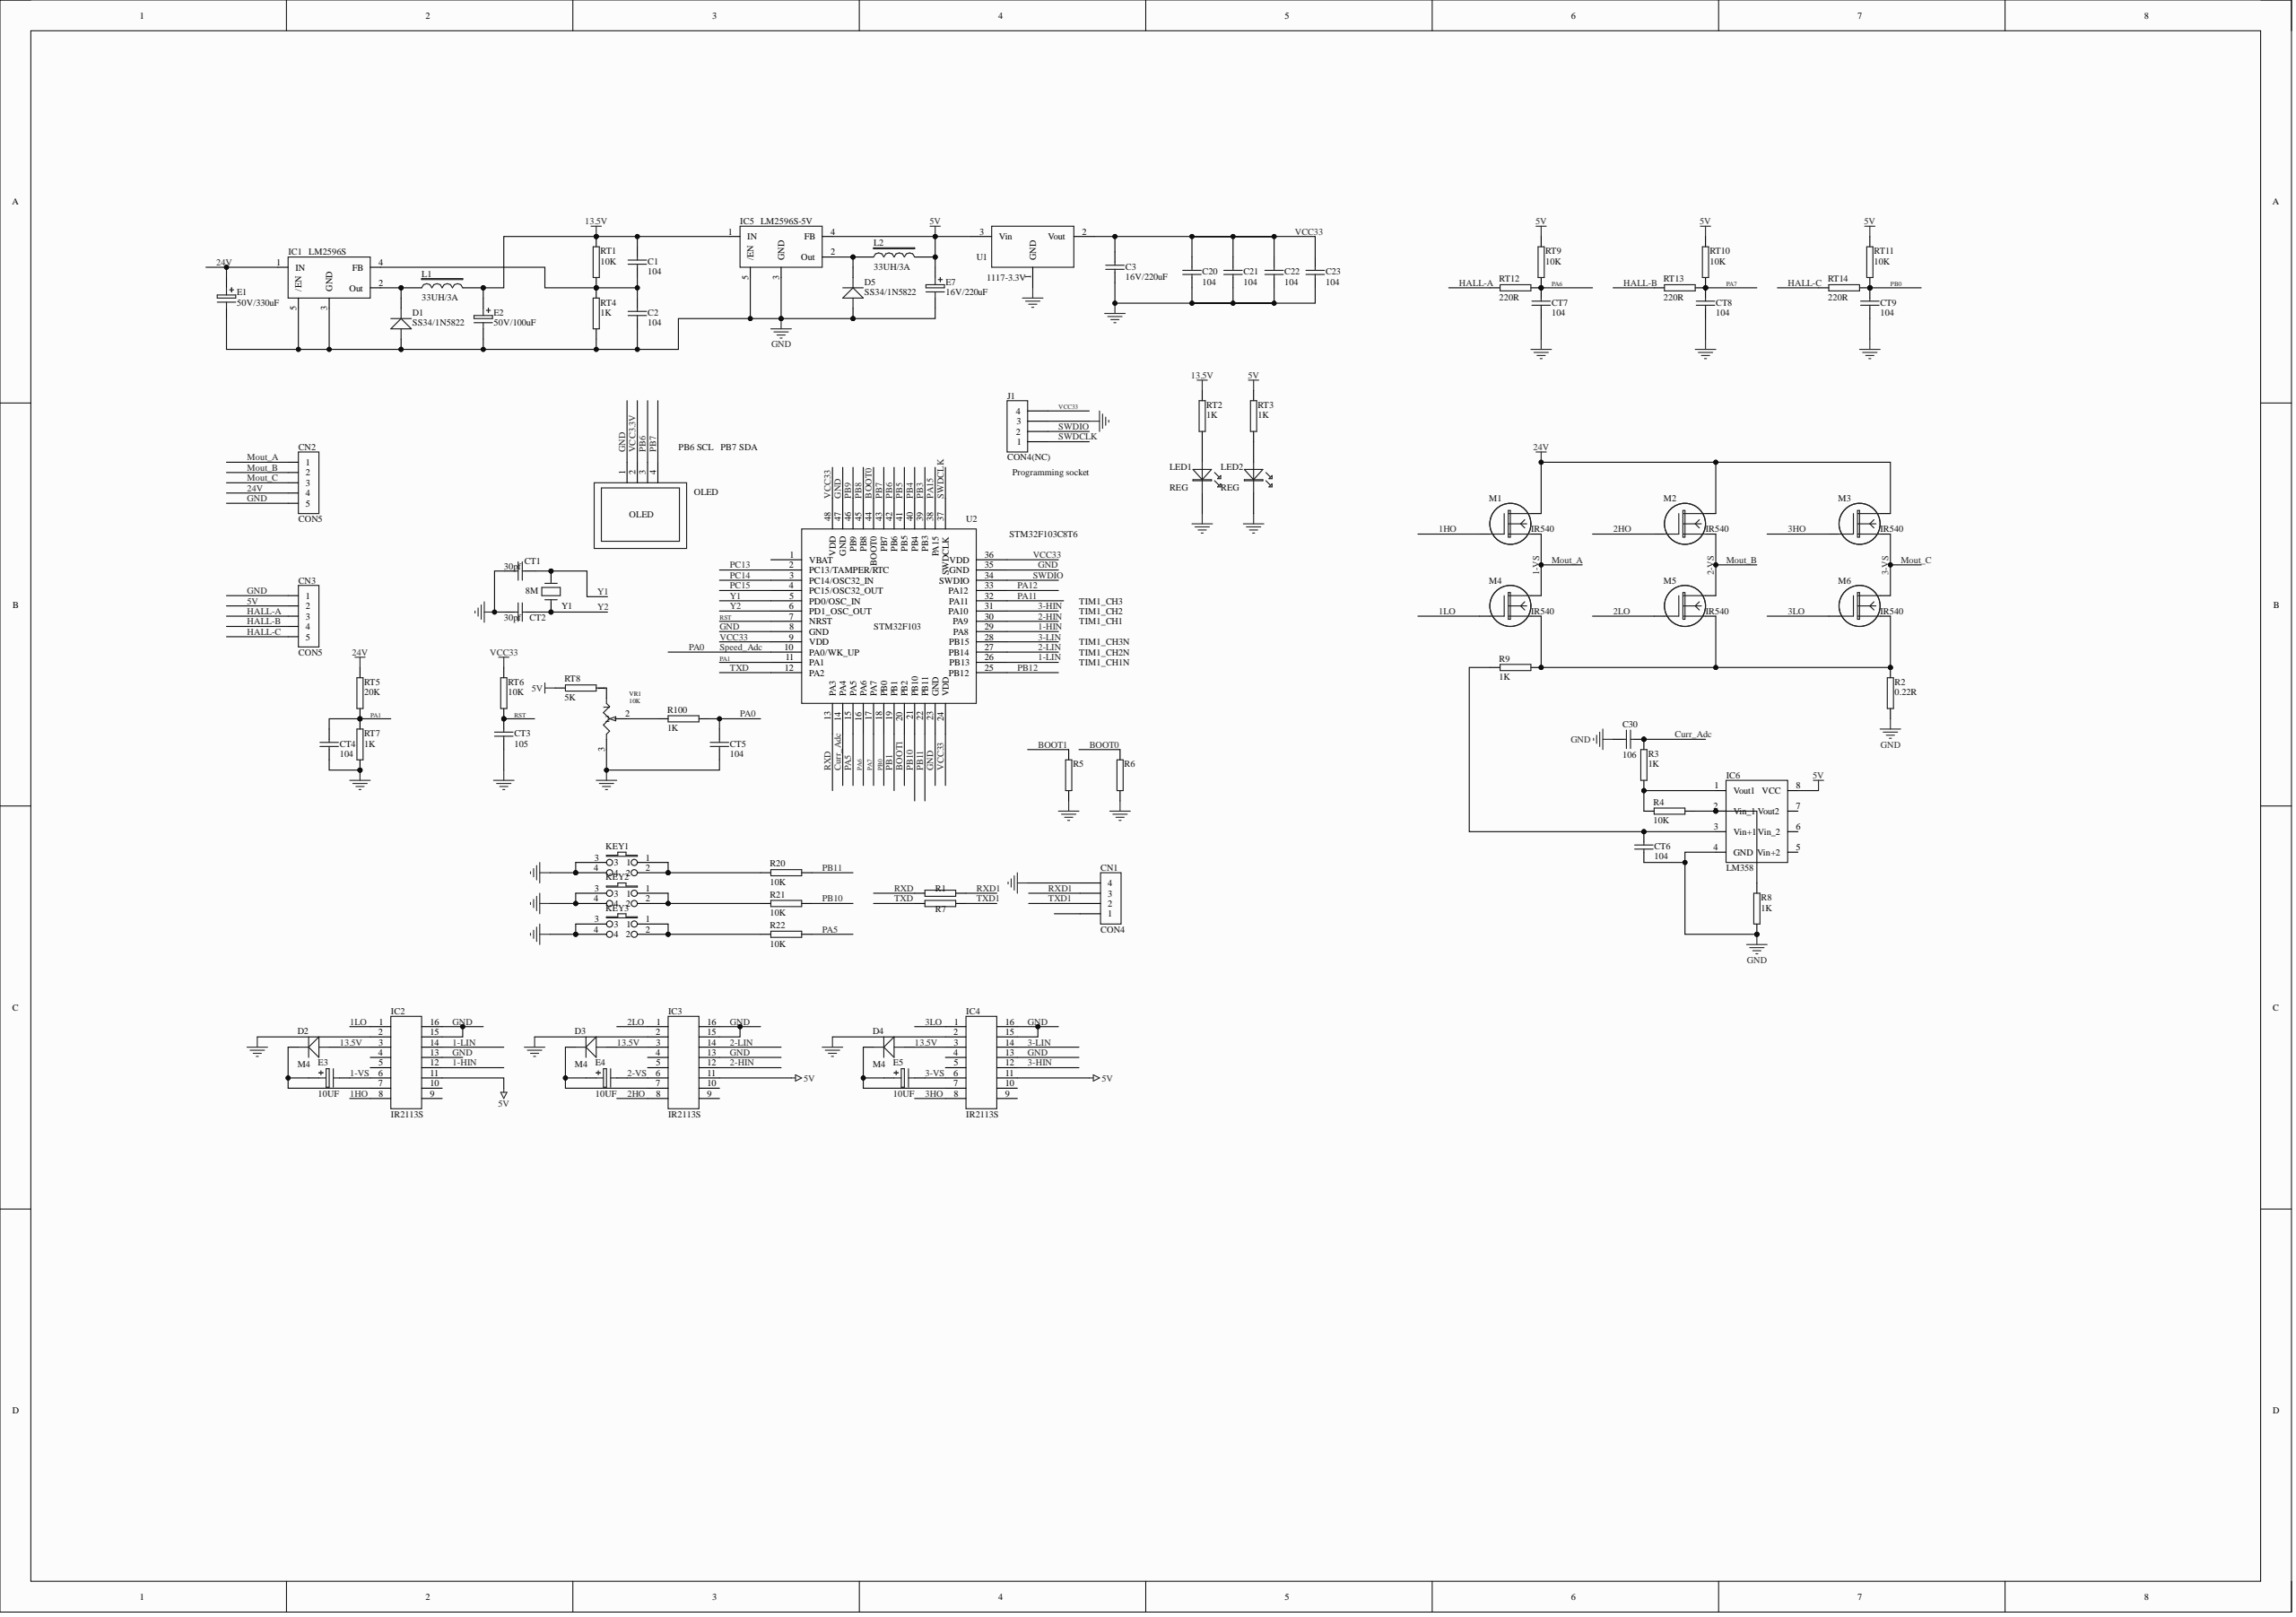Circuit board | Altium Designer | 83 parts | 62 nets
Bill of materials:
Comment,Description,Designator,Footprint,LibRef,Quantity
"104","Capacitor, [NoValue]","C1, C2, C20, C21, C22, C23, CT4, CT5, CT6, CT7, CT8, CT9","C0603","CAP, CAP_1","12"
"16V/220uF","Capacitor","C3","CAP-TH_BD5.0-P2.00-D0.8-FD-10UF50VC110GL","CAP","1"
"106","","C30","CAP-TH_BD5.0-P2.00-D0.8-FD-10UF50VC110GL","CAP_3","1"
"CON4","Connector","CN1","CON4","CON4_1","1"
"CON5","","CN2, CN3","CON5","CON5","2"
"30pf","","CT1, CT2","C0603","CAP_2, CAP_1","2"
"105","","CT3","C0603","CAP_1","1"
"SS34/1N5822","","D1, D5","SMA_L4.3-W2.5-LS5.0-RD","SS34/1N5822","2"
"M4","","D2, D3, D4","SMA_L4.3-W2.5-LS5.0-RD","SS34/1N5822","3"
"50V/330uF","","E1","50v/330uf","ELECTRO1","1"
"50V/100uF","","E2","50V/100UF","ELECTRO1","1"
"10UF","","E3, E4, E5","CAP-TH_BD5.0-P2.00-D0.8-FD-10UF50VC110GL","ELECTRO1, ELECTRO1_1","3"
"16V/220uF","","E7","16V/220UF","ELECTRO1","1"
"LM2596S","","IC1","LM2596S","LM2596S","1"
"IR2113S","","IC2, IC3, IC4","SOP-16","SOP-16","3"
"LM2596S-5V","","IC5","LM2596S","LM2596S","1"
"LM358","","IC6","lm358","HA17393","1"
"CON4(NC)","Connector","J1","HDR-TH_4P-P2.54-V-F","CON4","1"
"","","KEY1, KEY2, KEY3","SW-PB1","SW-PB1","3"
"33UH/3A","","L1, L2","IND-SMD_L11.5-W10.5_MWSA1004","INDUCTOR2","2"
"REG","","LED1, LED2","LED0603","LED","2"
"IR540","","M1, M2, M3, M4, M5, M6","IR5401","MOSFET-N1_QDZ","6"
"OLED","","OLED","OLED","OLED","1"
"100R","","R1, R7","R0603","RES2_3","2"
"0.22R","","R2","R0603","RES2_1","1"
"1K","","R3, R8, R9, R100, RT2, RT3, RT4, RT7","R0603","RES2_1, RES2_3, RES2","8"
"10K","","R4, R20, R21, R22, RT1, RT6, RT9, RT10, RT11","R0603","RES2_1, RES2_3, RES2","9"
"4.7K","","R5, R6","R0603","RES2_1","2"
"20K","","RT5","R0603","RES2","1"
"5K","","RT8","R0603","RES2_2","1"
"220R","","RT12, RT13, RT14","R0603","RES2_2","3"
"1117-3.3V","","U1","1117-3.3V","1117","1"
"STM32F103C8T6","","U2","STM32F103C8T6","STM32F103C8T6","1"
"10K","","VR1","R_3296","RES VAR 0932","1"
"8M","Crystal","Y1","HC-49S_L11.5-W5.0-P4.88","CRYSTAL","1"
Netlist (Protel format):
[
C1
C0603
104



]
[
C2
C0603
104



]
[
C3
CAP-TH_BD5.0-P2.00-D0.8-FD-10UF50VC110GL
16V/220uF



]
[
C20
C0603
104



]
[
C21
C0603
104



]
[
C22
C0603
104



]
[
C23
C0603
104



]
[
C30
CAP-TH_BD5.0-P2.00-D0.8-FD-10UF50VC110GL
106



]
[
CN1
CON4
CON4



]
[
CN2
CON5
CON5



]
[
CN3
CON5
CON5



]
[
CT1
C0603
30pf



]
[
CT2
C0603
30pf



]
[
CT3
C0603
105



]
[
CT4
C0603
104



]
[
CT5
C0603
104



]
[
CT6
C0603
104



]
[
CT7
C0603
104



]
[
CT8
C0603
104



]
[
CT9
C0603
104



]
[
D1
SMA_L4.3-W2.5-LS5.0-RD
SS34/1N5822



]
[
D2
SMA_L4.3-W2.5-LS5.0-RD
M4



]
[
D3
SMA_L4.3-W2.5-LS5.0-RD
M4



]
[
D4
SMA_L4.3-W2.5-LS5.0-RD
M4



]
[
D5
SMA_L4.3-W2.5-LS5.0-RD
SS34/1N5822



]
[
E1
50v/330uf
50V/330uF



]
[
E2
50V/100UF
50V/100uF



]
[
E3
CAP-TH_BD5.0-P2.00-D0.8-FD-10UF50VC110GL
10UF



]
[
E4
CAP-TH_BD5.0-P2.00-D0.8-FD-10UF50VC110GL
10UF



]
[
E5
CAP-TH_BD5.0-P2.00-D0.8-FD-10UF50VC110GL
10UF



]
[
E7
16V/220UF
16V/220uF



]
[
IC1
LM2596S
LM2596S



]
[
IC2
SOP-16
IR2113S



]
[
IC3
SOP-16
IR2113S



]
[
IC4
SOP-16
IR2113S



]
[
IC5
LM2596S
LM2596S-5V



]
[
IC6
lm358
LM358



]
[
J1
HDR-TH_4P-P2.54-V-F
CON4(NC)



]
[
KEY1
SW-PB1




]
[
KEY2
SW-PB1




]
[
KEY3
SW-PB1




]
[
L1
IND-SMD_L11.5-W10.5_MWSA1004
33UH/3A



]
[
L2
IND-SMD_L11.5-W10.5_MWSA1004
33UH/3A



]
[
LED1
LED0603
REG



]
[
LED2
LED0603
REG



]
[
M1
IR5401
IR540



]
[
M2
IR5401
IR540



]
[
M3
IR5401
IR540



]
[
M4
IR5401
IR540



]
[
M5
IR5401
IR540



]
[
M6
IR5401
IR540



]
[
OLED
OLED
OLED



]
[
R1
R0603
100R



]
[
R2
R0603
0.22R



]
[
R3
R0603
1K



]
[
R4
R0603
10K



]
[
R5
R0603
4.7K



]
[
R6
R0603
4.7K



]
[
R7
R0603
100R



]
[
R8
R0603
1K



]
[
R9
R0603
1K



]
[
R20
R0603
10K



]
[
R21
R0603
10K



]
[
R22
R0603
10K



]
[
R100
R0603
1K



]
[
RT1
R0603
10K



]
[
RT2
R0603
1K



]
[
RT3
R0603
1K



]
[
RT4
R0603
1K



]
[
RT5
R0603
20K



]
[
RT6
R0603
10K



]
[
RT7
R0603
1K



]
[
RT8
R0603
5K



]
[
RT9
R0603
10K



]
[
RT10
R0603
10K



]
[
RT11
R0603
10K



]
[
RT12
R0603
220R



]
[
RT13
R0603
220R



]
[
RT14
R0603
220R



]
[
U1
1117-3.3V
1117-3.3V



]
[
U2
STM32F103C8T6
STM32F103C8T6



]
[
VR1
R_3296
10K



]
[
Y1
HC-49S_L11.5-W5.0-P4.88
8M



]
(
Y2
CT2-2
U2-6
Y1-1
)
(
Y1
CT1-1
U2-5
Y1-2
)
(
VCC33
C3-1
C20-1
C21-1
C22-1
C23-1
J1-4
RT6-2
U1-2
U2-9
U2-24
U2-36
U2-48
)
(
TXD1
CN1-2
R7-1
)
(
TXD
R7-2
U2-12
)
(
SWDIO
J1-2
U2-34
)
(
SWDCLK
J1-1
U2-37
)
(
RXD1
CN1-3
R1-1
)
(
RXD
R1-2
U2-13
)
(
RST
CT3-2
RT6-1
U2-7
)
(
PB11
R20-1
U2-22
)
(
PB10
R21-1
U2-21
)
(
PB7
OLED-4
U2-43
)
(
PB6
OLED-3
U2-42
)
(
PB0
CT9-2
RT11-1
RT14-1
U2-18
)
(
PA7
CT8-2
RT10-1
RT13-1
U2-17
)
(
PA6
CT7-2
RT9-1
RT12-1
U2-16
)
(
PA5
R22-1
U2-15
)
(
PA1
CT4-2
RT5-1
RT7-2
U2-11
)
(
PA0
CT5-2
R100-1
U2-10
)
(
NetRT8_1
RT8-1
VR1-1
)
(
NetR100_2
R100-2
VR1-2
)
(
NetM4_3
M4-3
M5-3
M6-3
R2-1
R9-1
)
(
NetLED2_1
LED2-1
RT3-1
)
(
NetLED1_1
LED1-1
RT2-1
)
(
NetKEY3_1
KEY3-1
KEY3-2
R22-2
)
(
NetKEY2_1
KEY2-1
KEY2-2
R21-2
)
(
NetKEY1_1
KEY1-1
KEY1-2
R20-2
)
(
NetIC6_2
IC6-2
R4-1
R8-1
)
(
NetIC6_1
IC6-1
R3-2
R4-2
)
(
NetD5_1
D5-1
IC5-2
L2-1
)
(
NetD4_1
D4-1
E5-1
IC4-7
)
(
NetD3_1
D3-1
E4-1
IC3-7
)
(
NetD2_1
D2-1
E3-1
IC2-7
)
(
NetD1_1
D1-1
IC1-2
L1-1
)
(
NetCT6_2
CT6-2
IC6-3
R9-2
)
(
NetC1_2
C1-2
C2-1
IC1-4
RT1-1
RT4-2
)
(
HALL-C
CN3-5
RT14-2
)
(
HALL-B
CN3-4
RT13-2
)
(
HALL-A
CN3-3
RT12-2
)
(
GND
C2-2
C3-2
C20-2
C21-2
C22-2
C23-2
C30-2
CN2-5
CN3-1
CT1-2
CT2-1
CT3-1
CT4-1
CT5-1
CT6-1
CT7-1
CT8-1
CT9-1
D1-2
D5-2
E1-2
E2-2
E7-2
IC1-3
IC1-5
IC2-2
IC2-13
IC2-15
IC2-16
IC3-2
IC3-13
IC3-15
IC3-16
IC4-2
IC4-13
IC4-15
IC4-16
IC5-3
IC5-5
IC6-4
J1-3
KEY1-3
KEY1-4
KEY2-3
KEY2-4
KEY3-3
KEY3-4
LED1-2
LED2-2
OLED-1
R2-2
R5-1
R6-1
R8-2
RT4-1
RT7-1
U1-1
U2-8
U2-23
U2-35
U2-47
VR1-3
)
(
Curr_Adc
C30-1
R3-1
U2-14
)
(
BOOT1
R5-2
U2-20
)
(
BOOT0
R6-2
U2-44
)
(
24V
CN2-4
E1-1
IC1-1
M1-2
M2-2
M3-2
RT5-2
)
(
13.5V
C1-1
D2-2
D3-2
D4-2
E2-1
IC2-3
IC3-3
IC4-3
IC5-1
L1-2
RT1-2
RT2-2
)
(
5V
CN3-2
E7-1
IC2-11
IC3-11
IC4-11
IC5-4
IC6-8
L2-2
RT3-2
RT8-2
RT9-2
RT10-2
RT11-2
U1-3
)
(
3LO
IC4-1
M6-1
)
(
3HO
IC4-8
M3-1
)
(
3-VS
CN2-3
E5-2
IC4-6
M3-3
M6-2
)
(
3-LIN
IC4-14
U2-28
)
(
3-HIN
IC4-12
U2-31
)
(
2LO
IC3-1
M5-1
)
(
2HO
IC3-8
M2-1
)
(
2-VS
CN2-2
E4-2
IC3-6
M2-3
M5-2
)
(
2-LIN
IC3-14
U2-27
)
(
2-HIN
IC3-12
U2-30
)
(
1LO
IC2-1
M4-1
)
(
1HO
IC2-8
M1-1
)
(
1-VS
CN2-1
E3-2
IC2-6
M1-3
M4-2
)
(
1-LIN
IC2-14
U2-26
)
(
1-HIN
IC2-12
U2-29
)